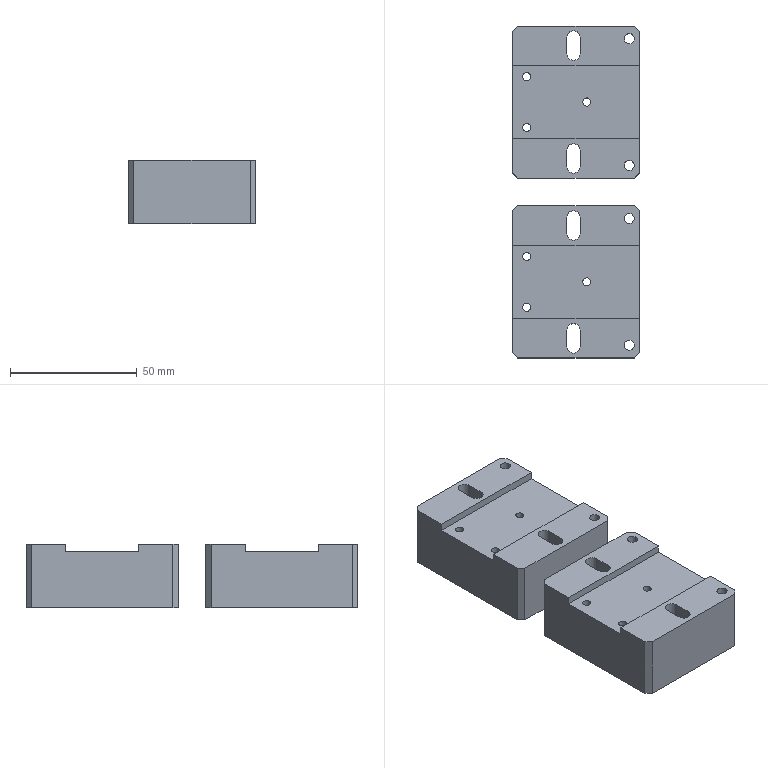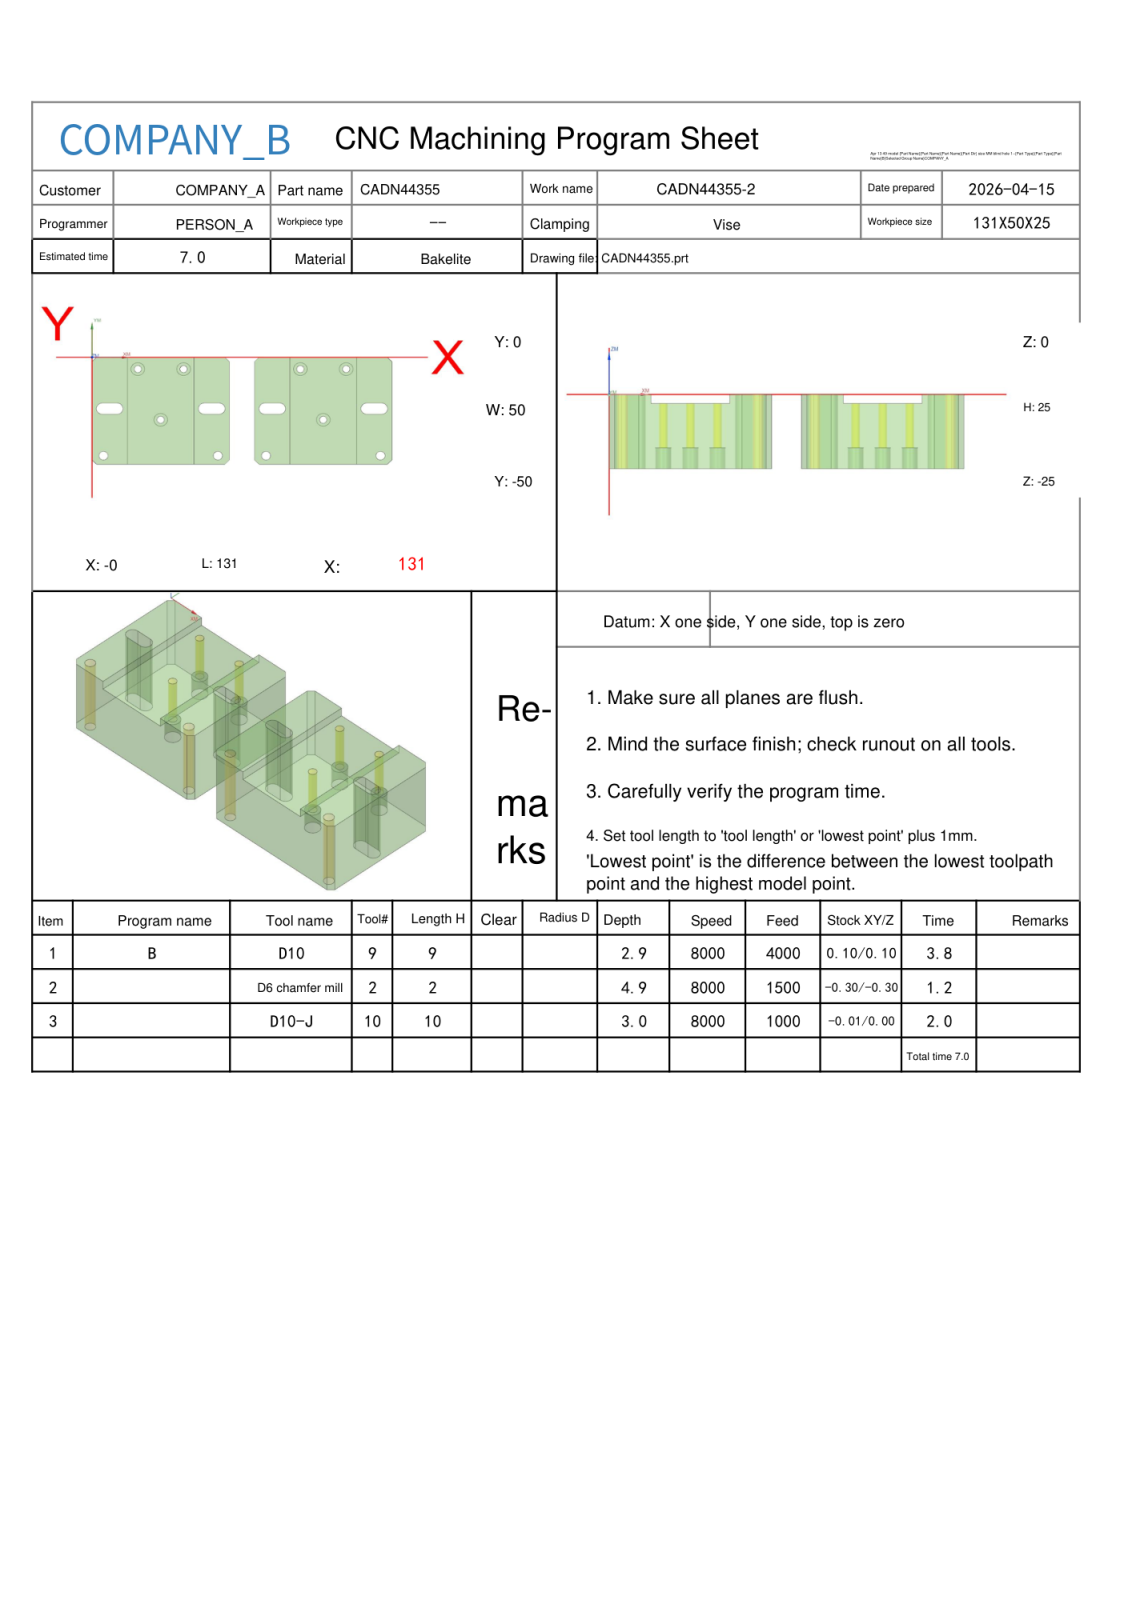NC program | NX | posted by the shop | part box 50 x 131 x 25 mm
Lines 3691 to 4338 of 4338:
N2 T02 M06
(D6 chamfer mill  D=6. R=0. H=02 ce=-0.30 di=0.00)
G00 G90 G54 X-.7 Y-10.954 M03 S7000
G43 H02 Z20.
M08
Z2.5
G01 Y-2.047 Z-.742 F1500.
X-.662 Y-1.84 Z-.819
X-.581 Y-1.645 Z-.895
X-.462 Y-1.472 Z-.972
X-.407 Y-1.417 Z-1.
X1.417 Y.407
G02 X2.124 Y.7 I.707 J-.707
G01 X15.15
G02 X16.15 Y-.3 I0.0 J-1.
G01 Y-49.7
G02 X15.15 Y-50.7 I-1. J0.0
G01 X2.124
G02 X1.417 Y-50.407 I0.0 J1.
G01 X-.407 Y-48.583
G02 X-.7 Y-47.876 I.707 J.707
G01 Y-2.124
G02 X-.407 Y-1.417 I1. J0.0
G01 X-.054 Y-1.064
Z1.5
G00 Z20.
X52.893 Y-50.7
Z2.5
G01 X44.772 Z-.456
X44.573 Y-50.664 Z-.529
X44.385 Y-50.589 Z-.603
X44.216 Y-50.477 Z-.677
X44.073 Y-50.334 Z-.751
X43.961 Y-50.165 Z-.824
X43.886 Y-49.977 Z-.898
X43.85 Y-49.778 Z-.972
Y-49.7 Z-1.
Y-.3
G02 X44.85 Y.7 I1. J0.0
G01 X57.876
G02 X58.583 Y.407 I0.0 J-1.
G01 X60.407 Y-1.417
G02 X60.7 Y-2.124 I-.707 J-.707
G01 Y-47.876
G02 X60.407 Y-48.583 I-1. J0.0
G01 X58.583 Y-50.407
G02 X57.876 Y-50.7 I-.707 J.707
G01 X44.85
G02 X43.85 Y-49.7 I0.0 J1.
G01 Y-49.2
Z1.5
G00 Z20.
X70.3 Y-10.954
Z2.5
G01 Y-2.047 Z-.742
X70.338 Y-1.84 Z-.819
X70.419 Y-1.645 Z-.895
X70.538 Y-1.472 Z-.972
X70.593 Y-1.417 Z-1.
X72.417 Y.407
G02 X73.124 Y.7 I.707 J-.707
G01 X86.15
G02 X87.15 Y-.3 I0.0 J-1.
G01 Y-49.7
G02 X86.15 Y-50.7 I-1. J0.0
G01 X73.124
G02 X72.417 Y-50.407 I0.0 J1.
G01 X70.593 Y-48.583
G02 X70.3 Y-47.876 I.707 J.707
G01 Y-2.124
G02 X70.593 Y-1.417 I1. J0.0
G01 X70.946 Y-1.064
Z1.5
G00 Z20.
X123.893 Y-50.7
Z2.5
G01 X115.772 Z-.456
X115.573 Y-50.664 Z-.529
X115.385 Y-50.589 Z-.603
X115.216 Y-50.477 Z-.677
X115.073 Y-50.334 Z-.751
X114.961 Y-50.165 Z-.824
X114.886 Y-49.977 Z-.898
X114.85 Y-49.778 Z-.972
Y-49.7 Z-1.
Y-.3
G02 X115.85 Y.7 I1. J0.0
G01 X128.876
G02 X129.583 Y.407 I0.0 J-1.
G01 X131.407 Y-1.417
G02 X131.7 Y-2.124 I-.707 J-.707
G01 Y-47.876
G02 X131.407 Y-48.583 I-1. J0.0
G01 X129.583 Y-50.407
G02 X128.876 Y-50.7 I-.707 J.707
G01 X115.85
G02 X114.85 Y-49.7 I0.0 J1.
G01 Y-49.2
Z1.5
G00 Z20.
G00 G90 X101. Y-29.2 M03 S8000
Z20.
G98 G81 X101. Y-29.2 Z-4.9 R0.0 F1000.
X111. Y-5.5
X91.
X40.
X20.
X30. Y-29.2
G80
G00 Z20.
G00 G90 X126. Y-46. M03 S8000
Z20.
G98 G81 X126. Y-46. Z-2.3 R3. F1000.
X76.
X55.
X5.
G80
G00 Z20.
G00 G90 X114.323 Y-25.386 M03 S6500
Z20.
Z.172
G01 Z-1.2 F1500.
G03 X114.523 Y-25.1 I-1.532 J1.286
G01 X114.553 Y-25.054
X114.55 Y-25.
Y0.0
G02 X115.55 Y1. I1. J0.0
G01 X129.
X129.259 Y.966
X129.5 Y.866
X129.707 Y.707
X131.707 Y-1.293
X131.866 Y-1.5
X131.966 Y-1.741
X132. Y-2.
Y-48.
X131.966 Y-48.259
X131.866 Y-48.5
X131.707 Y-48.707
X129.707 Y-50.707
X129.5 Y-50.866
X129.259 Y-50.966
X129. Y-51.
X115.55
G02 X114.55 Y-50. I0.0 J1.
G01 Y-25.
X114.553 Y-24.946
X114.523 Y-24.9
G03 X114.323 Y-24.614 I-1.732 J-1.
G01 Z.172
G00 Z10.
X126.412 Y-45.174
Z.33
G01 Z-1.2
G03 X126.103 Y-45.014 I-1.075 J-1.687
G01 X126.054 Y-44.99
X126. Y-45.
G03 X125. Y-46. I0.0 J-1.
X126. Y-47. I1. J0.0
X127. Y-46. I0.0 J1.
X126. Y-45. I-1. J0.0
G01 X125.946 Y-44.99
X125.897 Y-45.014
G03 X125.588 Y-45.174 I.765 J-1.848
G01 Z.33
G00 Z10.
X122.889 Y-25.373
Z.172
G01 Z-1.2
G03 X123.175 Y-25.573 I1.286 J1.532
G01 X123.221 Y-25.603
X123.275 Y-25.6
X126.5
G03 X128.1 Y-24. I0.0 J1.6
X126.5 Y-22.4 I-1.6 J0.0
G01 X120.05
G03 X118.45 Y-24. I0.0 J-1.6
X120.05 Y-25.6 I1.6 J0.0
G01 X123.275
X123.329 Y-25.603
X123.375 Y-25.573
G03 X123.661 Y-25.373 I-1. J1.732
G01 Z.172
G00 Z10.
X87.677 Y-24.614
Z.172
G01 Z-1.2
G03 X87.477 Y-24.9 I1.532 J-1.286
G01 X87.447 Y-24.946
X87.45 Y-25.
Y-50.
G02 X86.45 Y-51. I-1. J0.0
G01 X73.
X72.741 Y-50.966
X72.5 Y-50.866
X72.293 Y-50.707
X70.293 Y-48.707
X70.134 Y-48.5
X70.034 Y-48.259
X70. Y-48.
Y-2.
X70.034 Y-1.741
X70.134 Y-1.5
X70.293 Y-1.293
X72.293 Y.707
X72.5 Y.866
X72.741 Y.966
X73. Y1.
X86.45
G02 X87.45 Y0.0 I0.0 J-1.
G01 Y-25.
X87.447 Y-25.054
X87.477 Y-25.1
G03 X87.677 Y-25.386 I1.732 J1.
G01 Z.172
G00 Z2.55
X79.111 Y-22.627
Z.172
G01 Z-1.2
G03 X78.825 Y-22.427 I-1.286 J-1.532
G01 X78.779 Y-22.397
X78.725 Y-22.4
X75.5
G03 X73.9 Y-24. I0.0 J-1.6
X75.5 Y-25.6 I1.6 J0.0
G01 X81.95
G03 X83.55 Y-24. I0.0 J1.6
X81.95 Y-22.4 I-1.6 J0.0
G01 X78.725
X78.671 Y-22.397
X78.625 Y-22.427
G03 X78.339 Y-22.627 I1. J-1.732
G01 Z.172
G00 Z10.
X76.412 Y-45.174
Z.33
G01 Z-1.2
G03 X76.103 Y-45.014 I-1.075 J-1.687
G01 X76.054 Y-44.99
X76. Y-45.
G03 X75. Y-46. I0.0 J-1.
X76. Y-47. I1. J0.0
X77. Y-46. I0.0 J1.
X76. Y-45. I-1. J0.0
G01 X75.946 Y-44.99
X75.897 Y-45.014
G03 X75.588 Y-45.174 I.765 J-1.848
G01 Z.33
G00 Z10.
X61.227 Y-24.614
Z.172
G01 Z-1.2
G03 X61.027 Y-24.9 I1.532 J-1.286
G01 X60.997 Y-24.946
X61. Y-25.
Y-48.
X60.966 Y-48.259
X60.866 Y-48.5
X60.707 Y-48.707
X58.707 Y-50.707
X58.5 Y-50.866
X58.259 Y-50.966
X58. Y-51.
X44.55
G02 X43.55 Y-50. I0.0 J1.
G01 Y0.0
G02 X44.55 Y1. I1. J0.0
G01 X58.
X58.259 Y.966
X58.5 Y.866
X58.707 Y.707
X60.707 Y-1.293
X60.866 Y-1.5
X60.966 Y-1.741
X61. Y-2.
Y-25.
X60.997 Y-25.054
X61.027 Y-25.1
G03 X61.227 Y-25.386 I1.732 J1.
G01 Z.172
G00 Z10.
X55.412 Y-45.174
Z.33
G01 Z-1.2
G03 X55.103 Y-45.014 I-1.075 J-1.687
G01 X55.054 Y-44.99
X55. Y-45.
G03 X54. Y-46. I0.0 J-1.
X55. Y-47. I1. J0.0
X56. Y-46. I0.0 J1.
X55. Y-45. I-1. J0.0
G01 X54.946 Y-44.99
X54.897 Y-45.014
G03 X54.588 Y-45.174 I.765 J-1.848
G01 Z.33
G00 Z10.
X51.889 Y-25.373
Z.172
G01 Z-1.2
G03 X52.175 Y-25.573 I1.286 J1.532
G01 X52.221 Y-25.603
X52.275 Y-25.6
X55.5
G03 X57.1 Y-24. I0.0 J1.6
X55.5 Y-22.4 I-1.6 J0.0
G01 X49.05
G03 X47.45 Y-24. I0.0 J-1.6
X49.05 Y-25.6 I1.6 J0.0
G01 X52.275
X52.329 Y-25.603
X52.375 Y-25.573
G03 X52.661 Y-25.373 I-1. J1.732
G01 Z.172
G00 Z10.
X16.677 Y-24.614
Z.172
G01 Z-1.2
G03 X16.477 Y-24.9 I1.532 J-1.286
G01 X16.447 Y-24.946
X16.45 Y-25.
Y-50.
G02 X15.45 Y-51. I-1. J0.0
G01 X2.
X1.741 Y-50.966
X1.5 Y-50.866
X1.293 Y-50.707
X-.707 Y-48.707
X-.866 Y-48.5
X-.966 Y-48.259
X-1. Y-48.
Y-2.
X-.966 Y-1.741
X-.866 Y-1.5
X-.707 Y-1.293
X1.293 Y.707
X1.5 Y.866
X1.741 Y.966
X2. Y1.
X15.45
G02 X16.45 Y0.0 I0.0 J-1.
G01 Y-25.
X16.447 Y-25.054
X16.477 Y-25.1
G03 X16.677 Y-25.386 I1.732 J1.
G01 Z.172
G00 Z2.55
X7.339 Y-25.373
Z.172
G01 Z-1.2
G03 X7.625 Y-25.573 I1.286 J1.532
G01 X7.671 Y-25.603
X7.725 Y-25.6
X10.95
G03 X12.55 Y-24. I0.0 J1.6
X10.95 Y-22.4 I-1.6 J0.0
G01 X4.5
G03 X2.9 Y-24. I0.0 J-1.6
X4.5 Y-25.6 I1.6 J0.0
G01 X7.725
X7.779 Y-25.603
X7.825 Y-25.573
G03 X8.111 Y-25.373 I-1. J1.732
G01 Z.172
G00 Z10.
X5.412 Y-45.174
Z.33
G01 Z-1.2
G03 X5.103 Y-45.014 I-1.075 J-1.687
G01 X5.054 Y-44.99
X5. Y-45.
G03 X4. Y-46. I0.0 J-1.
X5. Y-47. I1. J0.0
X6. Y-46. I0.0 J1.
X5. Y-45. I-1. J0.0
G01 X4.946 Y-44.99
X4.897 Y-45.014
G03 X4.588 Y-45.174 I.765 J-1.848
G01 Z.33
G00 Z10.
X18.46 Y1.068
Z-1.795
G01 Z-4.2
X18.546 Y1.008
X18.576 Y1.
X41.424
X41.454 Y1.008
X41.54 Y1.068
Z-1.795
G00 Z10.
Y-51.068
Z-1.795
G01 Z-4.2
X41.454 Y-51.008
X41.424 Y-51.
X18.576
X18.546 Y-51.008
X18.46 Y-51.068
Z-1.795
G00 Z10.
X29.581 Y-29.644
Z-2.585
G01 Z-4.2
G03 X29.897 Y-29.791 I1. J1.732
G01 X29.947 Y-29.812
X30. Y-29.8
G03 X30.6 Y-29.2 I0.0 J.6
X30. Y-28.6 I-.6 J0.0
X29.4 Y-29.2 I0.0 J-.6
X30. Y-29.8 I.6 J0.0
G01 X30.053 Y-29.812
X30.103 Y-29.791
G03 X30.419 Y-29.644 I-.684 J1.879
G01 Z-2.585
G00 Z10.
X39.581 Y-5.944
Z-2.585
G01 Z-4.2
G03 X39.897 Y-6.091 I1. J1.732
G01 X39.947 Y-6.112
X40. Y-6.1
G03 X40.6 Y-5.5 I0.0 J.6
X40. Y-4.9 I-.6 J0.0
X39.4 Y-5.5 I0.0 J-.6
X40. Y-6.1 I.6 J0.0
G01 X40.053 Y-6.112
X40.103 Y-6.091
G03 X40.419 Y-5.944 I-.684 J1.879
G01 Z-2.127
G00 Z10.
X19.581
Z-2.127
G01 Z-4.2
G03 X19.897 Y-6.091 I1. J1.732
G01 X19.947 Y-6.112
X20. Y-6.1
G03 X20.6 Y-5.5 I0.0 J.6
X20. Y-4.9 I-.6 J0.0
X19.4 Y-5.5 I0.0 J-.6
X20. Y-6.1 I.6 J0.0
G01 X20.053 Y-6.112
X20.103 Y-6.091
G03 X20.419 Y-5.944 I-.684 J1.879
G01 Z-2.585
G00 Z10.
X112.54 Y-51.068
Z-1.795
G01 Z-4.2
X112.454 Y-51.008
X112.424 Y-51.
X89.576
X89.546 Y-51.008
X89.46 Y-51.068
Z-1.795
G00 Z10.
Y1.068
Z-1.795
G01 Z-4.2
X89.546 Y1.008
X89.576 Y1.
X112.424
X112.454 Y1.008
X112.54 Y1.068
Z-1.795
G00 Z10.
X100.581 Y-29.644
Z-2.585
G01 Z-4.2
G03 X100.897 Y-29.791 I1. J1.732
G01 X100.947 Y-29.812
X101. Y-29.8
G03 X101.6 Y-29.2 I0.0 J.6
X101. Y-28.6 I-.6 J0.0
X100.4 Y-29.2 I0.0 J-.6
X101. Y-29.8 I.6 J0.0
G01 X101.053 Y-29.812
X101.103 Y-29.791
G03 X101.419 Y-29.644 I-.684 J1.879
G01 Z-2.585
G00 Z10.
X90.581 Y-5.944
Z-2.127
G01 Z-4.2
G03 X90.897 Y-6.091 I1. J1.732
G01 X90.947 Y-6.112
X91. Y-6.1
G03 X91.6 Y-5.5 I0.0 J.6
X91. Y-4.9 I-.6 J0.0
X90.4 Y-5.5 I0.0 J-.6
X91. Y-6.1 I.6 J0.0
G01 X91.053 Y-6.112
X91.103 Y-6.091
G03 X91.419 Y-5.944 I-.684 J1.879
G01 Z-2.585
G00 Z10.
X110.581
Z-2.585
G01 Z-4.2
G03 X110.897 Y-6.091 I1. J1.732
G01 X110.947 Y-6.112
X111. Y-6.1
G03 X111.6 Y-5.5 I0.0 J.6
X111. Y-4.9 I-.6 J0.0
X110.4 Y-5.5 I0.0 J-.6
X111. Y-6.1 I.6 J0.0
G01 X111.053 Y-6.112
X111.103 Y-6.091
G03 X111.419 Y-5.944 I-.684 J1.879
G01 Z-2.127
G00 Z20.
G91 G28 Z0.0
M05
M09
G91 G28 Z0.0
M01
N3 T10 M06
(D10-J  D=10. R=0. H=10 ce=0.00 di=0.00)
G00 G90 G54 X-16.999 Y-3.001 M03 S8000
G43 H10 Z20.
M08
Z2.
G01 Z0.0 F1000.
X-4.999
X135.
G02 X135.999 Y-4. I-.001 J-1.
G01 Y-9.168
G02 X135. Y-10.167 I-1. J.001
G01 X-4.
G03 X-4.999 Y-11.167 I.001 J-1.
G01 Y-16.335
G03 X-4. Y-17.334 I1. J.001
G01 X135.
G02 X135.999 Y-18.333 I-.001 J-1.
G01 Y-23.501
G02 X135. Y-24.5 I-1. J.001
G01 X-4.
G03 X-4.999 Y-25.499 I.001 J-1.
G01 Y-30.667
G03 X-4. Y-31.666 I1. J.001
G01 X135.
G02 X135.999 Y-32.665 I-.001 J-1.
G01 Y-37.833
G02 X135. Y-38.833 I-1. J.001
G01 X-4.
G03 X-4.999 Y-39.832 I.001 J-1.
G01 Y-45.
G03 X-4. Y-45.999 I1. J.001
G01 X135.999
X147.999
Z2.
G00 Z20.
G00 G90 X37.149 Y7. M03 S8000
Z14.8
Z-1.5
G01 Z-3. F1000.
Y3.
G03 X39.149 Y5. I0.0 J2.
G01 Y-54.1
G02 X38.249 Y-55. I-.9 J0.0
G01 X35.574
G02 X34.574 Y-54. I0.0 J1.
G01 Y4.1
G03 X33.674 Y5. I-.9 J0.0
G01 X31.
G03 X30. Y4. I0.0 J-1.
G01 Y-54.1
G02 X29.1 Y-55. I-.9 J0.0
G01 X26.425
G02 X25.425 Y-54. I0.0 J1.
G01 Y4.1
G03 X24.525 Y5. I-.9 J0.0
G01 X21.85
G03 X20.85 Y4. I0.0 J-1.
G01 Y-55.
G03 X22.85 Y-57. I2. J0.0
G01 Z-1.5
G00 Z14.8
X108.149 Y7.
Z-1.5
G01 Z-3.
Y3.
G03 X110.149 Y5. I0.0 J2.
G01 Y-54.1
G02 X109.249 Y-55. I-.9 J0.0
G01 X106.574
G02 X105.574 Y-54. I0.0 J1.
G01 Y4.1
G03 X104.674 Y5. I-.9 J0.0
G01 X102.
G03 X101. Y4. I0.0 J-1.
G01 Y-54.1
G02 X100.1 Y-55. I-.9 J0.0
G01 X97.425
G02 X96.425 Y-54. I0.0 J1.
G01 Y4.1
G03 X95.525 Y5. I-.9 J0.0
G01 X92.85
G03 X91.85 Y4. I0.0 J-1.
G01 Y-55.
G03 X93.85 Y-57. I2. J0.0
G01 Z-1.5
G00 Z14.8
G00 G90 X37.611 Y-57.009 M03 S8000
Z14.8
Z-2.
G01 Z-3. F1000.
G41 D10
X37.809 Y-56.985
G03 X39.565 Y-55. I-.244 J1.985
G01 Y5.
G03 X37.809 Y6.985 I-2. J0.0
G01 G40 X37.611 Y7.009
Z-2.
G00 X22.389
G01 Z-3.
G41 D10
X22.191 Y6.985
G03 X20.435 Y5. I.244 J-1.985
G01 Y-55.
G03 X22.191 Y-56.985 I2. J0.0
G01 G40 X22.389 Y-57.009
Z-2.
G00 Z2.
X108.611
Z-2.
G01 Z-3.
G41 D10
X108.809 Y-56.985
G03 X110.565 Y-55. I-.244 J1.985
G01 Y5.
G03 X108.809 Y6.985 I-2. J0.0
G01 G40 X108.611 Y7.009
Z-2.
G00 X93.389
G01 Z-3.
G41 D10
X93.191 Y6.985
G03 X91.435 Y5. I.244 J-1.985
G01 Y-55.
G03 X93.191 Y-56.985 I2. J0.0
G01 G40 X93.389 Y-57.009
Z-2.
G00 Z14.8
M05
M09
G91 G28 Z0.0
G91 G28 Y0.0
M30
%